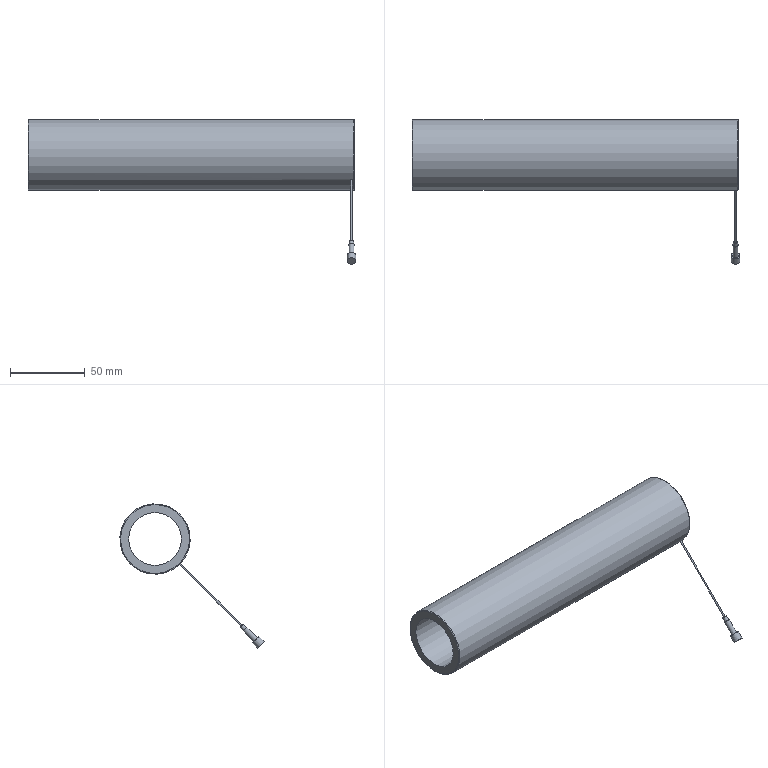Part | STEP file | Tube Heater_Bala35_toe | 1 solid | 14 faces | box 219 x 96.332 x 96.332 mm | volume 165765 mm3 | cylinder 6 | plane 6 | torus 2 | commonest cylinder face diameters 1 x1 3 x1 3.6 x1 6 x1 35.25 x1 47 x1